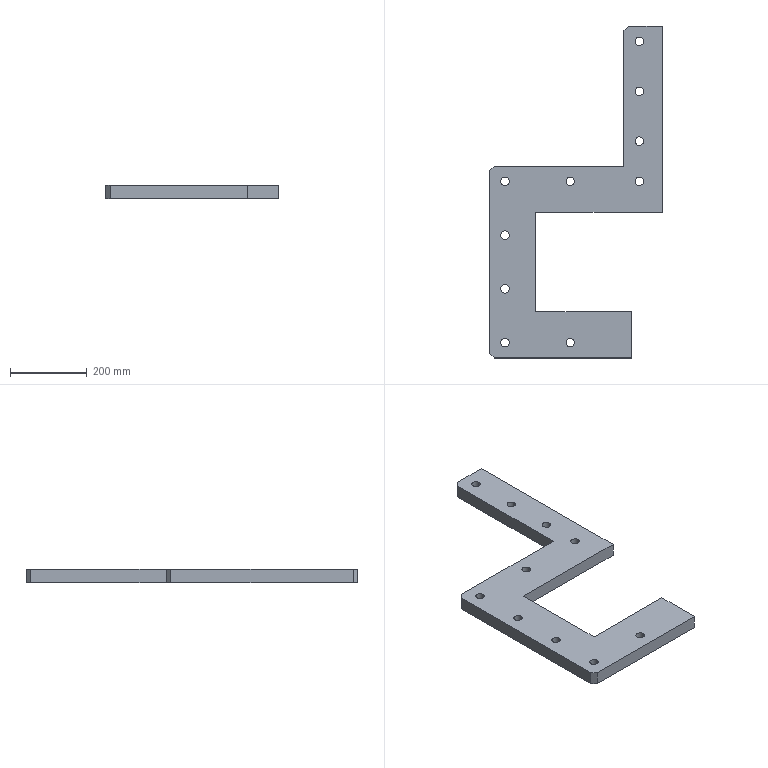Part | SolidWorks | features Chamfer 1, Extrusion 1, ICE 1 | 1 solid | 35 faces | box 450 x 865 x 35 mm | volume 5672894 mm3 | cylinder 20 | plane 15 | commonest cylinder face diameters 22 x20
STEP:
#1=CARTESIAN_POINT('',(-71.,-40.,0.));
#2=VERTEX_POINT('',#1);
#3=CARTESIAN_POINT('',(-49.,-40.,0.));
#4=VERTEX_POINT('',#3);
#5=CARTESIAN_POINT('',(-60.,-40.,0.));
#6=DIRECTION('',(0.,0.,1.));
#7=DIRECTION('',(1.,0.,0.));
#8=AXIS2_PLACEMENT_3D('',#5,#6,#7);
#9=CIRCLE('',#8,11.);
#10=EDGE_CURVE('',#2,#4,#9,.T.);
#11=ORIENTED_EDGE('',*,*,#10,.F.);
#12=CARTESIAN_POINT('',(-71.,-40.,35.));
#13=VERTEX_POINT('',#12);
#14=CARTESIAN_POINT('',(-71.,-40.,0.));
#15=DIRECTION('',(0.,0.,1.));
#16=VECTOR('',#15,1000.);
#17=LINE('',#14,#16);
#18=EDGE_CURVE('',#2,#13,#17,.T.);
#19=ORIENTED_EDGE('',*,*,#18,.T.);
#20=CARTESIAN_POINT('',(-49.,-40.,35.));
#21=VERTEX_POINT('',#20);
#22=CARTESIAN_POINT('',(-60.,-40.,35.));
#23=DIRECTION('',(0.,0.,1.));
#24=DIRECTION('',(1.,0.,0.));
#25=AXIS2_PLACEMENT_3D('',#22,#23,#24);
#26=CIRCLE('',#25,11.);
#27=EDGE_CURVE('',#13,#21,#26,.T.);
#28=ORIENTED_EDGE('',*,*,#27,.T.);
#29=CARTESIAN_POINT('',(-49.,-40.,0.));
#30=DIRECTION('',(0.,0.,1.));
#31=VECTOR('',#30,1000.);
#32=LINE('',#29,#31);
#33=EDGE_CURVE('',#4,#21,#32,.T.);
#34=ORIENTED_EDGE('',*,*,#33,.F.);
#35=EDGE_LOOP('',(#11,#19,#28,#34));
#36=FACE_OUTER_BOUND('',#35,.T.);
#37=CARTESIAN_POINT('',(-60.,-40.,0.));
#38=DIRECTION('',(0.,0.,1.));
#39=DIRECTION('',(1.,0.,0.));
#40=AXIS2_PLACEMENT_3D('',#37,#38,#39);
#41=CYLINDRICAL_SURFACE('',#40,11.);
#42=ADVANCED_FACE('',(#36),#41,.F.);
#43=CARTESIAN_POINT('',(-251.,-825.,0.));
#44=VERTEX_POINT('',#43);
#45=CARTESIAN_POINT('',(-229.,-825.,0.));
#46=VERTEX_POINT('',#45);
#47=CARTESIAN_POINT('',(-240.,-825.,0.));
#48=DIRECTION('',(0.,0.,1.));
#49=DIRECTION('',(1.,0.,0.));
#50=AXIS2_PLACEMENT_3D('',#47,#48,#49);
#51=CIRCLE('',#50,11.);
#52=EDGE_CURVE('',#44,#46,#51,.T.);
#53=ORIENTED_EDGE('',*,*,#52,.F.);
#54=CARTESIAN_POINT('',(-251.,-825.,35.));
#55=VERTEX_POINT('',#54);
#56=CARTESIAN_POINT('',(-251.,-825.,0.));
#57=DIRECTION('',(0.,0.,1.));
#58=VECTOR('',#57,1000.);
#59=LINE('',#56,#58);
#60=EDGE_CURVE('',#44,#55,#59,.T.);
#61=ORIENTED_EDGE('',*,*,#60,.T.);
#62=CARTESIAN_POINT('',(-229.,-825.,35.));
#63=VERTEX_POINT('',#62);
#64=CARTESIAN_POINT('',(-240.,-825.,35.));
#65=DIRECTION('',(0.,0.,1.));
#66=DIRECTION('',(1.,0.,0.));
#67=AXIS2_PLACEMENT_3D('',#64,#65,#66);
#68=CIRCLE('',#67,11.);
#69=EDGE_CURVE('',#55,#63,#68,.T.);
#70=ORIENTED_EDGE('',*,*,#69,.T.);
#71=CARTESIAN_POINT('',(-229.,-825.,0.));
#72=DIRECTION('',(0.,0.,1.));
#73=VECTOR('',#72,1000.);
#74=LINE('',#71,#73);
#75=EDGE_CURVE('',#46,#63,#74,.T.);
#76=ORIENTED_EDGE('',*,*,#75,.F.);
#77=EDGE_LOOP('',(#53,#61,#70,#76));
#78=FACE_OUTER_BOUND('',#77,.T.);
#79=CARTESIAN_POINT('',(-240.,-825.,0.));
#80=DIRECTION('',(0.,0.,1.));
#81=DIRECTION('',(1.,0.,0.));
#82=AXIS2_PLACEMENT_3D('',#79,#80,#81);
#83=CYLINDRICAL_SURFACE('',#82,11.);
#84=ADVANCED_FACE('',(#78),#83,.F.);
#85=CARTESIAN_POINT('',(-421.,-825.,0.));
#86=VERTEX_POINT('',#85);
#87=CARTESIAN_POINT('',(-399.,-825.,0.));
#88=VERTEX_POINT('',#87);
#89=CARTESIAN_POINT('',(-410.,-825.,0.));
#90=DIRECTION('',(0.,0.,1.));
#91=DIRECTION('',(1.,0.,0.));
#92=AXIS2_PLACEMENT_3D('',#89,#90,#91);
#93=CIRCLE('',#92,11.);
#94=EDGE_CURVE('',#86,#88,#93,.T.);
#95=ORIENTED_EDGE('',*,*,#94,.F.);
#96=CARTESIAN_POINT('',(-421.,-825.,35.));
#97=VERTEX_POINT('',#96);
#98=CARTESIAN_POINT('',(-421.,-825.,0.));
#99=DIRECTION('',(0.,0.,1.));
#100=VECTOR('',#99,1000.);
#101=LINE('',#98,#100);
#102=EDGE_CURVE('',#86,#97,#101,.T.);
#103=ORIENTED_EDGE('',*,*,#102,.T.);
#104=CARTESIAN_POINT('',(-399.,-825.,35.));
#105=VERTEX_POINT('',#104);
#106=CARTESIAN_POINT('',(-410.,-825.,35.));
#107=DIRECTION('',(0.,0.,1.));
#108=DIRECTION('',(1.,0.,0.));
#109=AXIS2_PLACEMENT_3D('',#106,#107,#108);
#110=CIRCLE('',#109,11.);
#111=EDGE_CURVE('',#97,#105,#110,.T.);
#112=ORIENTED_EDGE('',*,*,#111,.T.);
#113=CARTESIAN_POINT('',(-399.,-825.,0.));
#114=DIRECTION('',(0.,0.,1.));
#115=VECTOR('',#114,1000.);
#116=LINE('',#113,#115);
#117=EDGE_CURVE('',#88,#105,#116,.T.);
#118=ORIENTED_EDGE('',*,*,#117,.F.);
#119=EDGE_LOOP('',(#95,#103,#112,#118));
#120=FACE_OUTER_BOUND('',#119,.T.);
#121=CARTESIAN_POINT('',(-410.,-825.,0.));
#122=DIRECTION('',(0.,0.,1.));
#123=DIRECTION('',(1.,0.,0.));
#124=AXIS2_PLACEMENT_3D('',#121,#122,#123);
#125=CYLINDRICAL_SURFACE('',#124,11.);
#126=ADVANCED_FACE('',(#120),#125,.F.);
#127=CARTESIAN_POINT('',(-421.,-685.,0.));
#128=VERTEX_POINT('',#127);
#129=CARTESIAN_POINT('',(-399.,-685.,0.));
#130=VERTEX_POINT('',#129);
#131=CARTESIAN_POINT('',(-410.,-685.,0.));
#132=DIRECTION('',(0.,0.,1.));
#133=DIRECTION('',(1.,0.,0.));
#134=AXIS2_PLACEMENT_3D('',#131,#132,#133);
#135=CIRCLE('',#134,11.);
#136=EDGE_CURVE('',#128,#130,#135,.T.);
#137=ORIENTED_EDGE('',*,*,#136,.F.);
#138=CARTESIAN_POINT('',(-421.,-685.,35.));
#139=VERTEX_POINT('',#138);
#140=CARTESIAN_POINT('',(-421.,-685.,0.));
#141=DIRECTION('',(0.,0.,1.));
#142=VECTOR('',#141,1000.);
#143=LINE('',#140,#142);
#144=EDGE_CURVE('',#128,#139,#143,.T.);
#145=ORIENTED_EDGE('',*,*,#144,.T.);
#146=CARTESIAN_POINT('',(-399.,-685.,35.));
#147=VERTEX_POINT('',#146);
#148=CARTESIAN_POINT('',(-410.,-685.,35.));
#149=DIRECTION('',(0.,0.,1.));
#150=DIRECTION('',(1.,0.,0.));
#151=AXIS2_PLACEMENT_3D('',#148,#149,#150);
#152=CIRCLE('',#151,11.);
#153=EDGE_CURVE('',#139,#147,#152,.T.);
#154=ORIENTED_EDGE('',*,*,#153,.T.);
#155=CARTESIAN_POINT('',(-399.,-685.,0.));
#156=DIRECTION('',(0.,0.,1.));
#157=VECTOR('',#156,1000.);
#158=LINE('',#155,#157);
#159=EDGE_CURVE('',#130,#147,#158,.T.);
#160=ORIENTED_EDGE('',*,*,#159,.F.);
#161=EDGE_LOOP('',(#137,#145,#154,#160));
#162=FACE_OUTER_BOUND('',#161,.T.);
#163=CARTESIAN_POINT('',(-410.,-685.,0.));
#164=DIRECTION('',(0.,0.,1.));
#165=DIRECTION('',(1.,0.,0.));
#166=AXIS2_PLACEMENT_3D('',#163,#164,#165);
#167=CYLINDRICAL_SURFACE('',#166,11.);
#168=ADVANCED_FACE('',(#162),#167,.F.);
#169=CARTESIAN_POINT('',(-421.,-545.,0.));
#170=VERTEX_POINT('',#169);
#171=CARTESIAN_POINT('',(-399.,-545.,0.));
#172=VERTEX_POINT('',#171);
#173=CARTESIAN_POINT('',(-410.,-545.,0.));
#174=DIRECTION('',(0.,0.,1.));
#175=DIRECTION('',(1.,0.,0.));
#176=AXIS2_PLACEMENT_3D('',#173,#174,#175);
#177=CIRCLE('',#176,11.);
#178=EDGE_CURVE('',#170,#172,#177,.T.);
#179=ORIENTED_EDGE('',*,*,#178,.F.);
#180=CARTESIAN_POINT('',(-421.,-545.,35.));
#181=VERTEX_POINT('',#180);
#182=CARTESIAN_POINT('',(-421.,-545.,0.));
#183=DIRECTION('',(0.,0.,1.));
#184=VECTOR('',#183,1000.);
#185=LINE('',#182,#184);
#186=EDGE_CURVE('',#170,#181,#185,.T.);
#187=ORIENTED_EDGE('',*,*,#186,.T.);
#188=CARTESIAN_POINT('',(-399.,-545.,35.));
#189=VERTEX_POINT('',#188);
#190=CARTESIAN_POINT('',(-410.,-545.,35.));
#191=DIRECTION('',(0.,0.,1.));
#192=DIRECTION('',(1.,0.,0.));
#193=AXIS2_PLACEMENT_3D('',#190,#191,#192);
#194=CIRCLE('',#193,11.);
#195=EDGE_CURVE('',#181,#189,#194,.T.);
#196=ORIENTED_EDGE('',*,*,#195,.T.);
#197=CARTESIAN_POINT('',(-399.,-545.,0.));
#198=DIRECTION('',(0.,0.,1.));
#199=VECTOR('',#198,1000.);
#200=LINE('',#197,#199);
#201=EDGE_CURVE('',#172,#189,#200,.T.);
#202=ORIENTED_EDGE('',*,*,#201,.F.);
#203=EDGE_LOOP('',(#179,#187,#196,#202));
#204=FACE_OUTER_BOUND('',#203,.T.);
#205=CARTESIAN_POINT('',(-410.,-545.,0.));
#206=DIRECTION('',(0.,0.,1.));
#207=DIRECTION('',(1.,0.,0.));
#208=AXIS2_PLACEMENT_3D('',#205,#206,#207);
#209=CYLINDRICAL_SURFACE('',#208,11.);
#210=ADVANCED_FACE('',(#204),#209,.F.);
#211=CARTESIAN_POINT('',(-421.,-405.,0.));
#212=VERTEX_POINT('',#211);
#213=CARTESIAN_POINT('',(-399.,-405.,0.));
#214=VERTEX_POINT('',#213);
#215=CARTESIAN_POINT('',(-410.,-405.,0.));
#216=DIRECTION('',(0.,0.,1.));
#217=DIRECTION('',(1.,0.,0.));
#218=AXIS2_PLACEMENT_3D('',#215,#216,#217);
#219=CIRCLE('',#218,11.);
#220=EDGE_CURVE('',#212,#214,#219,.T.);
#221=ORIENTED_EDGE('',*,*,#220,.F.);
#222=CARTESIAN_POINT('',(-421.,-405.,35.));
#223=VERTEX_POINT('',#222);
#224=CARTESIAN_POINT('',(-421.,-405.,0.));
#225=DIRECTION('',(0.,0.,1.));
#226=VECTOR('',#225,1000.);
#227=LINE('',#224,#226);
#228=EDGE_CURVE('',#212,#223,#227,.T.);
#229=ORIENTED_EDGE('',*,*,#228,.T.);
#230=CARTESIAN_POINT('',(-399.,-405.,35.));
#231=VERTEX_POINT('',#230);
#232=CARTESIAN_POINT('',(-410.,-405.,35.));
#233=DIRECTION('',(0.,0.,1.));
#234=DIRECTION('',(1.,0.,0.));
#235=AXIS2_PLACEMENT_3D('',#232,#233,#234);
#236=CIRCLE('',#235,11.);
#237=EDGE_CURVE('',#223,#231,#236,.T.);
#238=ORIENTED_EDGE('',*,*,#237,.T.);
#239=CARTESIAN_POINT('',(-399.,-405.,0.));
#240=DIRECTION('',(0.,0.,1.));
#241=VECTOR('',#240,1000.);
#242=LINE('',#239,#241);
#243=EDGE_CURVE('',#214,#231,#242,.T.);
#244=ORIENTED_EDGE('',*,*,#243,.F.);
#245=EDGE_LOOP('',(#221,#229,#238,#244));
#246=FACE_OUTER_BOUND('',#245,.T.);
#247=CARTESIAN_POINT('',(-410.,-405.,0.));
#248=DIRECTION('',(0.,0.,1.));
#249=DIRECTION('',(1.,0.,0.));
#250=AXIS2_PLACEMENT_3D('',#247,#248,#249);
#251=CYLINDRICAL_SURFACE('',#250,11.);
#252=ADVANCED_FACE('',(#246),#251,.F.);
#253=CARTESIAN_POINT('',(-251.,-405.,0.));
#254=VERTEX_POINT('',#253);
#255=CARTESIAN_POINT('',(-229.,-405.,0.));
#256=VERTEX_POINT('',#255);
#257=CARTESIAN_POINT('',(-240.,-405.,0.));
#258=DIRECTION('',(0.,0.,1.));
#259=DIRECTION('',(1.,0.,0.));
#260=AXIS2_PLACEMENT_3D('',#257,#258,#259);
#261=CIRCLE('',#260,11.);
#262=EDGE_CURVE('',#254,#256,#261,.T.);
#263=ORIENTED_EDGE('',*,*,#262,.F.);
#264=CARTESIAN_POINT('',(-251.,-405.,35.));
#265=VERTEX_POINT('',#264);
#266=CARTESIAN_POINT('',(-251.,-405.,0.));
#267=DIRECTION('',(0.,0.,1.));
#268=VECTOR('',#267,1000.);
#269=LINE('',#266,#268);
#270=EDGE_CURVE('',#254,#265,#269,.T.);
#271=ORIENTED_EDGE('',*,*,#270,.T.);
#272=CARTESIAN_POINT('',(-229.,-405.,35.));
#273=VERTEX_POINT('',#272);
#274=CARTESIAN_POINT('',(-240.,-405.,35.));
#275=DIRECTION('',(0.,0.,1.));
#276=DIRECTION('',(1.,0.,0.));
#277=AXIS2_PLACEMENT_3D('',#274,#275,#276);
#278=CIRCLE('',#277,11.);
#279=EDGE_CURVE('',#265,#273,#278,.T.);
#280=ORIENTED_EDGE('',*,*,#279,.T.);
#281=CARTESIAN_POINT('',(-229.,-405.,0.));
#282=DIRECTION('',(0.,0.,1.));
#283=VECTOR('',#282,1000.);
#284=LINE('',#281,#283);
#285=EDGE_CURVE('',#256,#273,#284,.T.);
#286=ORIENTED_EDGE('',*,*,#285,.F.);
#287=EDGE_LOOP('',(#263,#271,#280,#286));
#288=FACE_OUTER_BOUND('',#287,.T.);
#289=CARTESIAN_POINT('',(-240.,-405.,0.));
#290=DIRECTION('',(0.,0.,1.));
#291=DIRECTION('',(1.,0.,0.));
#292=AXIS2_PLACEMENT_3D('',#289,#290,#291);
#293=CYLINDRICAL_SURFACE('',#292,11.);
#294=ADVANCED_FACE('',(#288),#293,.F.);
#295=CARTESIAN_POINT('',(-71.,-405.,0.));
#296=VERTEX_POINT('',#295);
#297=CARTESIAN_POINT('',(-49.,-405.,0.));
#298=VERTEX_POINT('',#297);
#299=CARTESIAN_POINT('',(-60.,-405.,0.));
#300=DIRECTION('',(0.,0.,1.));
#301=DIRECTION('',(1.,0.,0.));
#302=AXIS2_PLACEMENT_3D('',#299,#300,#301);
#303=CIRCLE('',#302,11.);
#304=EDGE_CURVE('',#296,#298,#303,.T.);
#305=ORIENTED_EDGE('',*,*,#304,.F.);
#306=CARTESIAN_POINT('',(-71.,-405.,35.));
#307=VERTEX_POINT('',#306);
#308=CARTESIAN_POINT('',(-71.,-405.,0.));
#309=DIRECTION('',(0.,0.,1.));
#310=VECTOR('',#309,1000.);
#311=LINE('',#308,#310);
#312=EDGE_CURVE('',#296,#307,#311,.T.);
#313=ORIENTED_EDGE('',*,*,#312,.T.);
#314=CARTESIAN_POINT('',(-49.,-405.,35.));
#315=VERTEX_POINT('',#314);
#316=CARTESIAN_POINT('',(-60.,-405.,35.));
#317=DIRECTION('',(0.,0.,1.));
#318=DIRECTION('',(1.,0.,0.));
#319=AXIS2_PLACEMENT_3D('',#316,#317,#318);
#320=CIRCLE('',#319,11.);
#321=EDGE_CURVE('',#307,#315,#320,.T.);
#322=ORIENTED_EDGE('',*,*,#321,.T.);
#323=CARTESIAN_POINT('',(-49.,-405.,0.));
#324=DIRECTION('',(0.,0.,1.));
#325=VECTOR('',#324,1000.);
#326=LINE('',#323,#325);
#327=EDGE_CURVE('',#298,#315,#326,.T.);
#328=ORIENTED_EDGE('',*,*,#327,.F.);
#329=EDGE_LOOP('',(#305,#313,#322,#328));
#330=FACE_OUTER_BOUND('',#329,.T.);
#331=CARTESIAN_POINT('',(-60.,-405.,0.));
#332=DIRECTION('',(0.,0.,1.));
#333=DIRECTION('',(1.,0.,0.));
#334=AXIS2_PLACEMENT_3D('',#331,#332,#333);
#335=CYLINDRICAL_SURFACE('',#334,11.);
#336=ADVANCED_FACE('',(#330),#335,.F.);
#337=CARTESIAN_POINT('',(-71.,-300.,0.));
#338=VERTEX_POINT('',#337);
#339=CARTESIAN_POINT('',(-49.,-300.,0.));
#340=VERTEX_POINT('',#339);
#341=CARTESIAN_POINT('',(-60.,-300.,0.));
#342=DIRECTION('',(0.,0.,1.));
#343=DIRECTION('',(1.,0.,0.));
#344=AXIS2_PLACEMENT_3D('',#341,#342,#343);
#345=CIRCLE('',#344,11.);
#346=EDGE_CURVE('',#338,#340,#345,.T.);
#347=ORIENTED_EDGE('',*,*,#346,.F.);
#348=CARTESIAN_POINT('',(-71.,-300.,35.));
#349=VERTEX_POINT('',#348);
#350=CARTESIAN_POINT('',(-71.,-300.,0.));
#351=DIRECTION('',(0.,0.,1.));
#352=VECTOR('',#351,1000.);
#353=LINE('',#350,#352);
#354=EDGE_CURVE('',#338,#349,#353,.T.);
#355=ORIENTED_EDGE('',*,*,#354,.T.);
#356=CARTESIAN_POINT('',(-49.,-300.,35.));
#357=VERTEX_POINT('',#356);
#358=CARTESIAN_POINT('',(-60.,-300.,35.));
#359=DIRECTION('',(0.,0.,1.));
#360=DIRECTION('',(1.,0.,0.));
#361=AXIS2_PLACEMENT_3D('',#358,#359,#360);
#362=CIRCLE('',#361,11.);
#363=EDGE_CURVE('',#349,#357,#362,.T.);
#364=ORIENTED_EDGE('',*,*,#363,.T.);
#365=CARTESIAN_POINT('',(-49.,-300.,0.));
#366=DIRECTION('',(0.,0.,1.));
#367=VECTOR('',#366,1000.);
#368=LINE('',#365,#367);
#369=EDGE_CURVE('',#340,#357,#368,.T.);
#370=ORIENTED_EDGE('',*,*,#369,.F.);
#371=EDGE_LOOP('',(#347,#355,#364,#370));
#372=FACE_OUTER_BOUND('',#371,.T.);
#373=CARTESIAN_POINT('',(-60.,-300.,0.));
#374=DIRECTION('',(0.,0.,1.));
#375=DIRECTION('',(1.,0.,0.));
#376=AXIS2_PLACEMENT_3D('',#373,#374,#375);
#377=CYLINDRICAL_SURFACE('',#376,11.);
#378=ADVANCED_FACE('',(#372),#377,.F.);
#379=CARTESIAN_POINT('',(-71.,-170.,0.));
#380=VERTEX_POINT('',#379);
#381=CARTESIAN_POINT('',(-49.,-170.,0.));
#382=VERTEX_POINT('',#381);
#383=CARTESIAN_POINT('',(-60.,-170.,0.));
#384=DIRECTION('',(0.,0.,1.));
#385=DIRECTION('',(1.,0.,0.));
#386=AXIS2_PLACEMENT_3D('',#383,#384,#385);
#387=CIRCLE('',#386,11.);
#388=EDGE_CURVE('',#380,#382,#387,.T.);
#389=ORIENTED_EDGE('',*,*,#388,.F.);
#390=CARTESIAN_POINT('',(-71.,-170.,35.));
#391=VERTEX_POINT('',#390);
#392=CARTESIAN_POINT('',(-71.,-170.,0.));
#393=DIRECTION('',(0.,0.,1.));
#394=VECTOR('',#393,1000.);
#395=LINE('',#392,#394);
#396=EDGE_CURVE('',#380,#391,#395,.T.);
#397=ORIENTED_EDGE('',*,*,#396,.T.);
#398=CARTESIAN_POINT('',(-49.,-170.,35.));
#399=VERTEX_POINT('',#398);
#400=CARTESIAN_POINT('',(-60.,-170.,35.));
#401=DIRECTION('',(0.,0.,1.));
#402=DIRECTION('',(1.,0.,0.));
#403=AXIS2_PLACEMENT_3D('',#400,#401,#402);
#404=CIRCLE('',#403,11.);
#405=EDGE_CURVE('',#391,#399,#404,.T.);
#406=ORIENTED_EDGE('',*,*,#405,.T.);
#407=CARTESIAN_POINT('',(-49.,-170.,0.));
#408=DIRECTION('',(0.,0.,1.));
#409=VECTOR('',#408,1000.);
#410=LINE('',#407,#409);
#411=EDGE_CURVE('',#382,#399,#410,.T.);
#412=ORIENTED_EDGE('',*,*,#411,.F.);
#413=EDGE_LOOP('',(#389,#397,#406,#412));
#414=FACE_OUTER_BOUND('',#413,.T.);
#415=CARTESIAN_POINT('',(-60.,-170.,0.));
#416=DIRECTION('',(0.,0.,1.));
#417=DIRECTION('',(1.,0.,0.));
#418=AXIS2_PLACEMENT_3D('',#415,#416,#417);
#419=CYLINDRICAL_SURFACE('',#418,11.);
#420=ADVANCED_FACE('',(#414),#419,.F.);
#421=CARTESIAN_POINT('',(-100.,-365.,0.));
#422=VERTEX_POINT('',#421);
#423=CARTESIAN_POINT('',(-438.,-365.,0.));
#424=VERTEX_POINT('',#423);
#425=CARTESIAN_POINT('',(-100.,-365.,0.));
#426=DIRECTION('',(-1.,0.,0.));
#427=VECTOR('',#426,1000.);
#428=LINE('',#425,#427);
#429=EDGE_CURVE('',#422,#424,#428,.T.);
#430=ORIENTED_EDGE('',*,*,#429,.T.);
#431=CARTESIAN_POINT('',(-438.,-365.,35.));
#432=VERTEX_POINT('',#431);
#433=CARTESIAN_POINT('',(-438.,-365.,35.));
#434=DIRECTION('',(0.,0.,1.));
#435=VECTOR('',#434,1000.);
#436=LINE('',#433,#435);
#437=EDGE_CURVE('',#424,#432,#436,.T.);
#438=ORIENTED_EDGE('',*,*,#437,.T.);
#439=CARTESIAN_POINT('',(-100.,-365.,35.));
#440=VERTEX_POINT('',#439);
#441=CARTESIAN_POINT('',(-100.,-365.,35.));
#442=DIRECTION('',(-1.,0.,0.));
#443=VECTOR('',#442,1000.);
#444=LINE('',#441,#443);
#445=EDGE_CURVE('',#440,#432,#444,.T.);
#446=ORIENTED_EDGE('',*,*,#445,.F.);
#447=CARTESIAN_POINT('',(-100.,-365.,35.));
#448=DIRECTION('',(0.,0.,-1.));
#449=VECTOR('',#448,1000.);
#450=LINE('',#447,#449);
#451=EDGE_CURVE('',#440,#422,#450,.T.);
#452=ORIENTED_EDGE('',*,*,#451,.T.);
#453=EDGE_LOOP('',(#430,#438,#446,#452));
#454=FACE_OUTER_BOUND('',#453,.T.);
#455=CARTESIAN_POINT('',(-100.,-365.,35.));
#456=DIRECTION('',(0.,-1.,0.));
#457=DIRECTION('',(1.,0.,0.));
#458=AXIS2_PLACEMENT_3D('',#455,#456,#457);
#459=PLANE('',#458);
#460=ADVANCED_FACE('',(#454),#459,.F.);
#461=CARTESIAN_POINT('',(-450.,-377.,0.));
#462=VERTEX_POINT('',#461);
#463=CARTESIAN_POINT('',(-450.,-853.,0.));
#464=VERTEX_POINT('',#463);
#465=CARTESIAN_POINT('',(-450.,-365.,0.));
#466=DIRECTION('',(0.,-1.,0.));
#467=VECTOR('',#466,1000.);
#468=LINE('',#465,#467);
#469=EDGE_CURVE('',#462,#464,#468,.T.);
#470=ORIENTED_EDGE('',*,*,#469,.T.);
#471=CARTESIAN_POINT('',(-450.,-853.,35.));
#472=VERTEX_POINT('',#471);
#473=CARTESIAN_POINT('',(-450.,-853.,35.));
#474=DIRECTION('',(0.,0.,1.));
#475=VECTOR('',#474,1000.);
#476=LINE('',#473,#475);
#477=EDGE_CURVE('',#464,#472,#476,.T.);
#478=ORIENTED_EDGE('',*,*,#477,.T.);
#479=CARTESIAN_POINT('',(-450.,-377.,35.));
#480=VERTEX_POINT('',#479);
#481=CARTESIAN_POINT('',(-450.,-365.,35.));
#482=DIRECTION('',(0.,-1.,0.));
#483=VECTOR('',#482,1000.);
#484=LINE('',#481,#483);
#485=EDGE_CURVE('',#480,#472,#484,.T.);
#486=ORIENTED_EDGE('',*,*,#485,.F.);
#487=CARTESIAN_POINT('',(-450.,-377.,35.));
#488=DIRECTION('',(0.,0.,-1.));
#489=VECTOR('',#488,1000.);
#490=LINE('',#487,#489);
#491=EDGE_CURVE('',#480,#462,#490,.T.);
#492=ORIENTED_EDGE('',*,*,#491,.T.);
#493=EDGE_LOOP('',(#470,#478,#486,#492));
#494=FACE_OUTER_BOUND('',#493,.T.);
#495=CARTESIAN_POINT('',(-450.,-365.,35.));
#496=DIRECTION('',(1.,0.,0.));
#497=DIRECTION('',(0.,1.,0.));
#498=AXIS2_PLACEMENT_3D('',#495,#496,#497);
#499=PLANE('',#498);
#500=ADVANCED_FACE('',(#494),#499,.F.);
#501=CARTESIAN_POINT('',(-438.,-865.,35.));
#502=VERTEX_POINT('',#501);
#503=CARTESIAN_POINT('',(-80.,-865.,35.));
#504=VERTEX_POINT('',#503);
#505=CARTESIAN_POINT('',(-450.,-865.,35.));
#506=DIRECTION('',(1.,0.,0.));
#507=VECTOR('',#506,1000.);
#508=LINE('',#505,#507);
#509=EDGE_CURVE('',#502,#504,#508,.T.);
#510=ORIENTED_EDGE('',*,*,#509,.F.);
#511=CARTESIAN_POINT('',(-438.,-865.,0.));
#512=VERTEX_POINT('',#511);
#513=CARTESIAN_POINT('',(-438.,-865.,35.));
#514=DIRECTION('',(0.,0.,-1.));
#515=VECTOR('',#514,1000.);
#516=LINE('',#513,#515);
#517=EDGE_CURVE('',#502,#512,#516,.T.);
#518=ORIENTED_EDGE('',*,*,#517,.T.);
#519=CARTESIAN_POINT('',(-80.,-865.,0.));
#520=VERTEX_POINT('',#519);
#521=CARTESIAN_POINT('',(-450.,-865.,0.));
#522=DIRECTION('',(1.,0.,0.));
#523=VECTOR('',#522,1000.);
#524=LINE('',#521,#523);
#525=EDGE_CURVE('',#512,#520,#524,.T.);
#526=ORIENTED_EDGE('',*,*,#525,.T.);
#527=CARTESIAN_POINT('',(-80.,-865.,35.));
#528=DIRECTION('',(0.,0.,-1.));
#529=VECTOR('',#528,1000.);
#530=LINE('',#527,#529);
#531=EDGE_CURVE('',#504,#520,#530,.T.);
#532=ORIENTED_EDGE('',*,*,#531,.F.);
#533=EDGE_LOOP('',(#510,#518,#526,#532));
#534=FACE_OUTER_BOUND('',#533,.T.);
#535=CARTESIAN_POINT('',(-450.,-865.,35.));
#536=DIRECTION('',(0.,1.,0.));
#537=DIRECTION('',(0.,0.,1.));
#538=AXIS2_PLACEMENT_3D('',#535,#536,#537);
#539=PLANE('',#538);
#540=ADVANCED_FACE('',(#534),#539,.F.);
#541=CARTESIAN_POINT('',(-80.,-745.,0.));
#542=VERTEX_POINT('',#541);
#543=CARTESIAN_POINT('',(-80.,-865.,0.));
#544=DIRECTION('',(0.,1.,0.));
#545=VECTOR('',#544,1000.);
#546=LINE('',#543,#545);
#547=EDGE_CURVE('',#520,#542,#546,.T.);
#548=ORIENTED_EDGE('',*,*,#547,.T.);
#549=CARTESIAN_POINT('',(-80.,-745.,35.));
#550=VERTEX_POINT('',#549);
#551=CARTESIAN_POINT('',(-80.,-745.,35.));
#552=DIRECTION('',(0.,0.,-1.));
#553=VECTOR('',#552,1000.);
#554=LINE('',#551,#553);
#555=EDGE_CURVE('',#550,#542,#554,.T.);
#556=ORIENTED_EDGE('',*,*,#555,.F.);
#557=CARTESIAN_POINT('',(-80.,-865.,35.));
#558=DIRECTION('',(0.,1.,0.));
#559=VECTOR('',#558,1000.);
#560=LINE('',#557,#559);
#561=EDGE_CURVE('',#504,#550,#560,.T.);
#562=ORIENTED_EDGE('',*,*,#561,.F.);
#563=ORIENTED_EDGE('',*,*,#531,.T.);
#564=EDGE_LOOP('',(#548,#556,#562,#563));
#565=FACE_OUTER_BOUND('',#564,.T.);
#566=CARTESIAN_POINT('',(-80.,-865.,35.));
#567=DIRECTION('',(-1.,0.,0.));
#568=DIRECTION('',(0.,0.,1.));
#569=AXIS2_PLACEMENT_3D('',#566,#567,#568);
#570=PLANE('',#569);
#571=ADVANCED_FACE('',(#565),#570,.F.);
#572=CARTESIAN_POINT('',(-330.,-745.,0.));
#573=VERTEX_POINT('',#572);
#574=CARTESIAN_POINT('',(-330.,-745.,0.));
#575=DIRECTION('',(-1.,0.,0.));
#576=VECTOR('',#575,1000.);
#577=LINE('',#574,#576);
#578=EDGE_CURVE('',#542,#573,#577,.T.);
#579=ORIENTED_EDGE('',*,*,#578,.T.);
#580=CARTESIAN_POINT('',(-330.,-745.,35.));
#581=VERTEX_POINT('',#580);
#582=CARTESIAN_POINT('',(-330.,-745.,35.));
#583=DIRECTION('',(0.,0.,-1.));
#584=VECTOR('',#583,1000.);
#585=LINE('',#582,#584);
#586=EDGE_CURVE('',#581,#573,#585,.T.);
#587=ORIENTED_EDGE('',*,*,#586,.F.);
#588=CARTESIAN_POINT('',(-330.,-745.,35.));
#589=DIRECTION('',(-1.,0.,0.));
#590=VECTOR('',#589,1000.);
#591=LINE('',#588,#590);
#592=EDGE_CURVE('',#550,#581,#591,.T.);
#593=ORIENTED_EDGE('',*,*,#592,.F.);
#594=ORIENTED_EDGE('',*,*,#555,.T.);
#595=EDGE_LOOP('',(#579,#587,#593,#594));
#596=FACE_OUTER_BOUND('',#595,.T.);
#597=CARTESIAN_POINT('',(-330.,-745.,35.));
#598=DIRECTION('',(0.,-1.,0.));
#599=DIRECTION('',(0.,0.,-1.));
#600=AXIS2_PLACEMENT_3D('',#597,#598,#599);
#601=PLANE('',#600);
#602=ADVANCED_FACE('',(#596),#601,.F.);
#603=CARTESIAN_POINT('',(-330.,-485.,0.));
#604=VERTEX_POINT('',#603);
#605=CARTESIAN_POINT('',(-330.,-485.,0.));
#606=DIRECTION('',(0.,1.,0.));
#607=VECTOR('',#606,1000.);
#608=LINE('',#605,#607);
#609=EDGE_CURVE('',#573,#604,#608,.T.);
#610=ORIENTED_EDGE('',*,*,#609,.T.);
#611=CARTESIAN_POINT('',(-330.,-485.,35.));
#612=VERTEX_POINT('',#611);
#613=CARTESIAN_POINT('',(-330.,-485.,35.));
#614=DIRECTION('',(0.,0.,-1.));
#615=VECTOR('',#614,1000.);
#616=LINE('',#613,#615);
#617=EDGE_CURVE('',#612,#604,#616,.T.);
#618=ORIENTED_EDGE('',*,*,#617,.F.);
#619=CARTESIAN_POINT('',(-330.,-485.,35.));
#620=DIRECTION('',(0.,1.,0.));
#621=VECTOR('',#620,1000.);
#622=LINE('',#619,#621);
#623=EDGE_CURVE('',#581,#612,#622,.T.);
#624=ORIENTED_EDGE('',*,*,#623,.F.);
#625=ORIENTED_EDGE('',*,*,#586,.T.);
#626=EDGE_LOOP('',(#610,#618,#624,#625));
#627=FACE_OUTER_BOUND('',#626,.T.);
#628=CARTESIAN_POINT('',(-330.,-485.,35.));
#629=DIRECTION('',(-1.,0.,0.));
#630=DIRECTION('',(0.,-1.,0.));
#631=AXIS2_PLACEMENT_3D('',#628,#629,#630);
#632=PLANE('',#631);
#633=ADVANCED_FACE('',(#627),#632,.F.);
#634=CARTESIAN_POINT('',(0.,-485.,0.));
#635=VERTEX_POINT('',#634);
#636=CARTESIAN_POINT('',(0.,-485.,0.));
#637=DIRECTION('',(1.,0.,0.));
#638=VECTOR('',#637,1000.);
#639=LINE('',#636,#638);
#640=EDGE_CURVE('',#604,#635,#639,.T.);
#641=ORIENTED_EDGE('',*,*,#640,.T.);
#642=CARTESIAN_POINT('',(0.,-485.,35.));
#643=VERTEX_POINT('',#642);
#644=CARTESIAN_POINT('',(0.,-485.,35.));
#645=DIRECTION('',(0.,0.,-1.));
#646=VECTOR('',#645,1000.);
#647=LINE('',#644,#646);
#648=EDGE_CURVE('',#643,#635,#647,.T.);
#649=ORIENTED_EDGE('',*,*,#648,.F.);
#650=CARTESIAN_POINT('',(0.,-485.,35.));
#651=DIRECTION('',(1.,0.,0.));
#652=VECTOR('',#651,1000.);
#653=LINE('',#650,#652);
#654=EDGE_CURVE('',#612,#643,#653,.T.);
#655=ORIENTED_EDGE('',*,*,#654,.F.);
#656=ORIENTED_EDGE('',*,*,#617,.T.);
#657=EDGE_LOOP('',(#641,#649,#655,#656));
#658=FACE_OUTER_BOUND('',#657,.T.);
#659=CARTESIAN_POINT('',(0.,-485.,35.));
#660=DIRECTION('',(0.,1.,0.));
#661=DIRECTION('',(-1.,0.,0.));
#662=AXIS2_PLACEMENT_3D('',#659,#660,#661);
#663=PLANE('',#662);
#664=ADVANCED_FACE('',(#658),#663,.F.);
#665=CARTESIAN_POINT('',(0.,0.,0.));
#666=VERTEX_POINT('',#665);
#667=CARTESIAN_POINT('',(0.,0.,0.));
#668=DIRECTION('',(0.,1.,0.));
#669=VECTOR('',#668,1000.);
#670=LINE('',#667,#669);
#671=EDGE_CURVE('',#635,#666,#670,.T.);
#672=ORIENTED_EDGE('',*,*,#671,.T.);
#673=CARTESIAN_POINT('',(0.,0.,35.));
#674=VERTEX_POINT('',#673);
#675=CARTESIAN_POINT('',(0.,0.,35.));
#676=DIRECTION('',(0.,0.,-1.));
#677=VECTOR('',#676,1000.);
#678=LINE('',#675,#677);
#679=EDGE_CURVE('',#674,#666,#678,.T.);
#680=ORIENTED_EDGE('',*,*,#679,.F.);
#681=CARTESIAN_POINT('',(0.,0.,35.));
#682=DIRECTION('',(0.,1.,0.));
#683=VECTOR('',#682,1000.);
#684=LINE('',#681,#683);
#685=EDGE_CURVE('',#643,#674,#684,.T.);
#686=ORIENTED_EDGE('',*,*,#685,.F.);
#687=ORIENTED_EDGE('',*,*,#648,.T.);
#688=EDGE_LOOP('',(#672,#680,#686,#687));
#689=FACE_OUTER_BOUND('',#688,.T.);
#690=CARTESIAN_POINT('',(0.,0.,35.));
#691=DIRECTION('',(-1.,0.,0.));
#692=DIRECTION('',(0.,-1.,0.));
#693=AXIS2_PLACEMENT_3D('',#690,#691,#692);
#694=PLANE('',#693);
#695=ADVANCED_FACE('',(#689),#694,.F.);
#696=CARTESIAN_POINT('',(-88.,0.,0.));
#697=VERTEX_POINT('',#696);
#698=CARTESIAN_POINT('',(0.,0.,0.));
#699=DIRECTION('',(-1.,0.,0.));
#700=VECTOR('',#699,1000.);
#701=LINE('',#698,#700);
#702=EDGE_CURVE('',#666,#697,#701,.T.);
#703=ORIENTED_EDGE('',*,*,#702,.T.);
#704=CARTESIAN_POINT('',(-88.,0.,35.));
#705=VERTEX_POINT('',#704);
#706=CARTESIAN_POINT('',(-88.,0.,35.));
#707=DIRECTION('',(0.,0.,1.));
#708=VECTOR('',#707,1000.);
#709=LINE('',#706,#708);
#710=EDGE_CURVE('',#697,#705,#709,.T.);
#711=ORIENTED_EDGE('',*,*,#710,.T.);
#712=CARTESIAN_POINT('',(0.,0.,35.));
#713=DIRECTION('',(-1.,0.,0.));
#714=VECTOR('',#713,1000.);
#715=LINE('',#712,#714);
#716=EDGE_CURVE('',#674,#705,#715,.T.);
#717=ORIENTED_EDGE('',*,*,#716,.F.);
#718=ORIENTED_EDGE('',*,*,#679,.T.);
#719=EDGE_LOOP('',(#703,#711,#717,#718));
#720=FACE_OUTER_BOUND('',#719,.T.);
#721=CARTESIAN_POINT('',(0.,0.,35.));
#722=DIRECTION('',(0.,-1.,0.));
#723=DIRECTION('',(0.,0.,-1.));
#724=AXIS2_PLACEMENT_3D('',#721,#722,#723);
#725=PLANE('',#724);
#726=ADVANCED_FACE('',(#720),#725,.F.);
#727=CARTESIAN_POINT('',(-100.,-12.,35.));
#728=VERTEX_POINT('',#727);
#729=CARTESIAN_POINT('',(-100.,0.,35.));
#730=DIRECTION('',(0.,-1.,0.));
#731=VECTOR('',#730,1000.);
#732=LINE('',#729,#731);
#733=EDGE_CURVE('',#728,#440,#732,.T.);
#734=ORIENTED_EDGE('',*,*,#733,.F.);
#735=CARTESIAN_POINT('',(-100.,-12.,0.));
#736=VERTEX_POINT('',#735);
#737=CARTESIAN_POINT('',(-100.,-12.,35.));
#738=DIRECTION('',(0.,0.,-1.));
#739=VECTOR('',#738,1000.);
#740=LINE('',#737,#739);
#741=EDGE_CURVE('',#728,#736,#740,.T.);
#742=ORIENTED_EDGE('',*,*,#741,.T.);
#743=CARTESIAN_POINT('',(-100.,0.,0.));
#744=DIRECTION('',(0.,-1.,0.));
#745=VECTOR('',#744,1000.);
#746=LINE('',#743,#745);
#747=EDGE_CURVE('',#736,#422,#746,.T.);
#748=ORIENTED_EDGE('',*,*,#747,.T.);
#749=ORIENTED_EDGE('',*,*,#451,.F.);
#750=EDGE_LOOP('',(#734,#742,#748,#749));
#751=FACE_OUTER_BOUND('',#750,.T.);
#752=CARTESIAN_POINT('',(-100.,0.,35.));
#753=DIRECTION('',(1.,0.,0.));
#754=DIRECTION('',(0.,1.,0.));
#755=AXIS2_PLACEMENT_3D('',#752,#753,#754);
#756=PLANE('',#755);
#757=ADVANCED_FACE('',(#751),#756,.F.);
#758=CARTESIAN_POINT('',(-60.,-40.,35.));
#759=DIRECTION('',(0.,0.,1.));
#760=DIRECTION('',(1.,0.,0.));
#761=AXIS2_PLACEMENT_3D('',#758,#759,#760);
#762=CIRCLE('',#761,11.);
#763=EDGE_CURVE('',#21,#13,#762,.T.);
#764=ORIENTED_EDGE('',*,*,#763,.F.);
#765=ORIENTED_EDGE('',*,*,#27,.F.);
#766=EDGE_LOOP('',(#764,#765));
#767=FACE_BOUND('',#766,.T.);
#768=CARTESIAN_POINT('',(-240.,-825.,35.));
#769=DIRECTION('',(0.,0.,1.));
#770=DIRECTION('',(1.,0.,0.));
#771=AXIS2_PLACEMENT_3D('',#768,#769,#770);
#772=CIRCLE('',#771,11.);
#773=EDGE_CURVE('',#63,#55,#772,.T.);
#774=ORIENTED_EDGE('',*,*,#773,.F.);
#775=ORIENTED_EDGE('',*,*,#69,.F.);
#776=EDGE_LOOP('',(#774,#775));
#777=FACE_BOUND('',#776,.T.);
#778=CARTESIAN_POINT('',(-410.,-825.,35.));
#779=DIRECTION('',(0.,0.,1.));
#780=DIRECTION('',(1.,0.,0.));
#781=AXIS2_PLACEMENT_3D('',#778,#779,#780);
#782=CIRCLE('',#781,11.);
#783=EDGE_CURVE('',#105,#97,#782,.T.);
#784=ORIENTED_EDGE('',*,*,#783,.F.);
#785=ORIENTED_EDGE('',*,*,#111,.F.);
#786=EDGE_LOOP('',(#784,#785));
#787=FACE_BOUND('',#786,.T.);
#788=CARTESIAN_POINT('',(-410.,-685.,35.));
#789=DIRECTION('',(0.,0.,1.));
#790=DIRECTION('',(1.,0.,0.));
#791=AXIS2_PLACEMENT_3D('',#788,#789,#790);
#792=CIRCLE('',#791,11.);
#793=EDGE_CURVE('',#147,#139,#792,.T.);
#794=ORIENTED_EDGE('',*,*,#793,.F.);
#795=ORIENTED_EDGE('',*,*,#153,.F.);
#796=EDGE_LOOP('',(#794,#795));
#797=FACE_BOUND('',#796,.T.);
#798=CARTESIAN_POINT('',(-410.,-545.,35.));
#799=DIRECTION('',(0.,0.,1.));
#800=DIRECTION('',(1.,0.,0.));
#801=AXIS2_PLACEMENT_3D('',#798,#799,#800);
#802=CIRCLE('',#801,11.);
#803=EDGE_CURVE('',#189,#181,#802,.T.);
#804=ORIENTED_EDGE('',*,*,#803,.F.);
#805=ORIENTED_EDGE('',*,*,#195,.F.);
#806=EDGE_LOOP('',(#804,#805));
#807=FACE_BOUND('',#806,.T.);
#808=CARTESIAN_POINT('',(-410.,-405.,35.));
#809=DIRECTION('',(0.,0.,1.));
#810=DIRECTION('',(1.,0.,0.));
#811=AXIS2_PLACEMENT_3D('',#808,#809,#810);
#812=CIRCLE('',#811,11.);
#813=EDGE_CURVE('',#231,#223,#812,.T.);
#814=ORIENTED_EDGE('',*,*,#813,.F.);
#815=ORIENTED_EDGE('',*,*,#237,.F.);
#816=EDGE_LOOP('',(#814,#815));
#817=FACE_BOUND('',#816,.T.);
#818=CARTESIAN_POINT('',(-240.,-405.,35.));
#819=DIRECTION('',(0.,0.,1.));
#820=DIRECTION('',(1.,0.,0.));
#821=AXIS2_PLACEMENT_3D('',#818,#819,#820);
#822=CIRCLE('',#821,11.);
#823=EDGE_CURVE('',#273,#265,#822,.T.);
#824=ORIENTED_EDGE('',*,*,#823,.F.);
#825=ORIENTED_EDGE('',*,*,#279,.F.);
#826=EDGE_LOOP('',(#824,#825));
#827=FACE_BOUND('',#826,.T.);
#828=CARTESIAN_POINT('',(-60.,-405.,35.));
#829=DIRECTION('',(0.,0.,1.));
#830=DIRECTION('',(1.,0.,0.));
#831=AXIS2_PLACEMENT_3D('',#828,#829,#830);
#832=CIRCLE('',#831,11.);
#833=EDGE_CURVE('',#315,#307,#832,.T.);
#834=ORIENTED_EDGE('',*,*,#833,.F.);
#835=ORIENTED_EDGE('',*,*,#321,.F.);
#836=EDGE_LOOP('',(#834,#835));
#837=FACE_BOUND('',#836,.T.);
#838=CARTESIAN_POINT('',(-60.,-300.,35.));
#839=DIRECTION('',(0.,0.,1.));
#840=DIRECTION('',(1.,0.,0.));
#841=AXIS2_PLACEMENT_3D('',#838,#839,#840);
#842=CIRCLE('',#841,11.);
#843=EDGE_CURVE('',#357,#349,#842,.T.);
#844=ORIENTED_EDGE('',*,*,#843,.F.);
#845=ORIENTED_EDGE('',*,*,#363,.F.);
#846=EDGE_LOOP('',(#844,#845));
#847=FACE_BOUND('',#846,.T.);
#848=CARTESIAN_POINT('',(-60.,-170.,35.));
#849=DIRECTION('',(0.,0.,1.));
#850=DIRECTION('',(1.,0.,0.));
#851=AXIS2_PLACEMENT_3D('',#848,#849,#850);
#852=CIRCLE('',#851,11.);
#853=EDGE_CURVE('',#399,#391,#852,.T.);
#854=ORIENTED_EDGE('',*,*,#853,.F.);
#855=ORIENTED_EDGE('',*,*,#405,.F.);
#856=EDGE_LOOP('',(#854,#855));
#857=FACE_BOUND('',#856,.T.);
#858=ORIENTED_EDGE('',*,*,#485,.T.);
#859=CARTESIAN_POINT('',(-651.5,-651.5,35.));
#860=DIRECTION('',(0.7071,-0.7071,0.));
#861=VECTOR('',#860,1000.);
#862=LINE('',#859,#861);
#863=EDGE_CURVE('',#472,#502,#862,.T.);
#864=ORIENTED_EDGE('',*,*,#863,.T.);
#865=ORIENTED_EDGE('',*,*,#509,.T.);
#866=ORIENTED_EDGE('',*,*,#561,.T.);
#867=ORIENTED_EDGE('',*,*,#592,.T.);
#868=ORIENTED_EDGE('',*,*,#623,.T.);
#869=ORIENTED_EDGE('',*,*,#654,.T.);
#870=ORIENTED_EDGE('',*,*,#685,.T.);
#871=ORIENTED_EDGE('',*,*,#716,.T.);
#872=CARTESIAN_POINT('',(-44.,44.,35.));
#873=DIRECTION('',(-0.7071,-0.7071,0.));
#874=VECTOR('',#873,1000.);
#875=LINE('',#872,#874);
#876=EDGE_CURVE('',#705,#728,#875,.T.);
#877=ORIENTED_EDGE('',*,*,#876,.T.);
#878=ORIENTED_EDGE('',*,*,#733,.T.);
#879=ORIENTED_EDGE('',*,*,#445,.T.);
#880=CARTESIAN_POINT('',(-36.5,36.5,35.));
#881=DIRECTION('',(-0.7071,-0.7071,0.));
#882=VECTOR('',#881,1000.);
#883=LINE('',#880,#882);
#884=EDGE_CURVE('',#432,#480,#883,.T.);
#885=ORIENTED_EDGE('',*,*,#884,.T.);
#886=EDGE_LOOP('',(#858,#864,#865,#866,#867,#868,#869,#870,#871,#877,#878,#879,#885));
#887=FACE_OUTER_BOUND('',#886,.T.);
#888=CARTESIAN_POINT('',(0.,0.,35.));
#889=DIRECTION('',(0.,0.,1.));
#890=DIRECTION('',(1.,0.,0.));
#891=AXIS2_PLACEMENT_3D('',#888,#889,#890);
#892=PLANE('',#891);
#893=ADVANCED_FACE('',(#767,#777,#787,#797,#807,#817,#827,#837,#847,#857,#887),#892,.T.);
#894=CARTESIAN_POINT('',(-60.,-40.,0.));
#895=DIRECTION('',(0.,0.,1.));
#896=DIRECTION('',(1.,0.,0.));
#897=AXIS2_PLACEMENT_3D('',#894,#895,#896);
#898=CIRCLE('',#897,11.);
#899=EDGE_CURVE('',#4,#2,#898,.T.);
#900=ORIENTED_EDGE('',*,*,#899,.T.);
#901=ORIENTED_EDGE('',*,*,#10,.T.);
#902=EDGE_LOOP('',(#900,#901));
#903=FACE_BOUND('',#902,.T.);
#904=CARTESIAN_POINT('',(-240.,-825.,0.));
#905=DIRECTION('',(0.,0.,1.));
#906=DIRECTION('',(1.,0.,0.));
#907=AXIS2_PLACEMENT_3D('',#904,#905,#906);
#908=CIRCLE('',#907,11.);
#909=EDGE_CURVE('',#46,#44,#908,.T.);
#910=ORIENTED_EDGE('',*,*,#909,.T.);
#911=ORIENTED_EDGE('',*,*,#52,.T.);
#912=EDGE_LOOP('',(#910,#911));
#913=FACE_BOUND('',#912,.T.);
#914=CARTESIAN_POINT('',(-410.,-825.,0.));
#915=DIRECTION('',(0.,0.,1.));
#916=DIRECTION('',(1.,0.,0.));
#917=AXIS2_PLACEMENT_3D('',#914,#915,#916);
#918=CIRCLE('',#917,11.);
#919=EDGE_CURVE('',#88,#86,#918,.T.);
#920=ORIENTED_EDGE('',*,*,#919,.T.);
#921=ORIENTED_EDGE('',*,*,#94,.T.);
#922=EDGE_LOOP('',(#920,#921));
#923=FACE_BOUND('',#922,.T.);
#924=CARTESIAN_POINT('',(-410.,-685.,0.));
#925=DIRECTION('',(0.,0.,1.));
#926=DIRECTION('',(1.,0.,0.));
#927=AXIS2_PLACEMENT_3D('',#924,#925,#926);
#928=CIRCLE('',#927,11.);
#929=EDGE_CURVE('',#130,#128,#928,.T.);
#930=ORIENTED_EDGE('',*,*,#929,.T.);
#931=ORIENTED_EDGE('',*,*,#136,.T.);
#932=EDGE_LOOP('',(#930,#931));
#933=FACE_BOUND('',#932,.T.);
#934=CARTESIAN_POINT('',(-410.,-545.,0.));
#935=DIRECTION('',(0.,0.,1.));
#936=DIRECTION('',(1.,0.,0.));
#937=AXIS2_PLACEMENT_3D('',#934,#935,#936);
#938=CIRCLE('',#937,11.);
#939=EDGE_CURVE('',#172,#170,#938,.T.);
#940=ORIENTED_EDGE('',*,*,#939,.T.);
#941=ORIENTED_EDGE('',*,*,#178,.T.);
#942=EDGE_LOOP('',(#940,#941));
#943=FACE_BOUND('',#942,.T.);
#944=CARTESIAN_POINT('',(-410.,-405.,0.));
#945=DIRECTION('',(0.,0.,1.));
#946=DIRECTION('',(1.,0.,0.));
#947=AXIS2_PLACEMENT_3D('',#944,#945,#946);
#948=CIRCLE('',#947,11.);
#949=EDGE_CURVE('',#214,#212,#948,.T.);
#950=ORIENTED_EDGE('',*,*,#949,.T.);
#951=ORIENTED_EDGE('',*,*,#220,.T.);
#952=EDGE_LOOP('',(#950,#951));
#953=FACE_BOUND('',#952,.T.);
#954=CARTESIAN_POINT('',(-240.,-405.,0.));
#955=DIRECTION('',(0.,0.,1.));
#956=DIRECTION('',(1.,0.,0.));
#957=AXIS2_PLACEMENT_3D('',#954,#955,#956);
#958=CIRCLE('',#957,11.);
#959=EDGE_CURVE('',#256,#254,#958,.T.);
#960=ORIENTED_EDGE('',*,*,#959,.T.);
#961=ORIENTED_EDGE('',*,*,#262,.T.);
#962=EDGE_LOOP('',(#960,#961));
#963=FACE_BOUND('',#962,.T.);
#964=CARTESIAN_POINT('',(-60.,-405.,0.));
#965=DIRECTION('',(0.,0.,1.));
#966=DIRECTION('',(1.,0.,0.));
#967=AXIS2_PLACEMENT_3D('',#964,#965,#966);
#968=CIRCLE('',#967,11.);
#969=EDGE_CURVE('',#298,#296,#968,.T.);
#970=ORIENTED_EDGE('',*,*,#969,.T.);
#971=ORIENTED_EDGE('',*,*,#304,.T.);
#972=EDGE_LOOP('',(#970,#971));
#973=FACE_BOUND('',#972,.T.);
#974=CARTESIAN_POINT('',(-60.,-300.,0.));
#975=DIRECTION('',(0.,0.,1.));
#976=DIRECTION('',(1.,0.,0.));
#977=AXIS2_PLACEMENT_3D('',#974,#975,#976);
#978=CIRCLE('',#977,11.);
#979=EDGE_CURVE('',#340,#338,#978,.T.);
#980=ORIENTED_EDGE('',*,*,#979,.T.);
#981=ORIENTED_EDGE('',*,*,#346,.T.);
#982=EDGE_LOOP('',(#980,#981));
#983=FACE_BOUND('',#982,.T.);
#984=CARTESIAN_POINT('',(-60.,-170.,0.));
#985=DIRECTION('',(0.,0.,1.));
#986=DIRECTION('',(1.,0.,0.));
#987=AXIS2_PLACEMENT_3D('',#984,#985,#986);
#988=CIRCLE('',#987,11.);
#989=EDGE_CURVE('',#382,#380,#988,.T.);
#990=ORIENTED_EDGE('',*,*,#989,.T.);
#991=ORIENTED_EDGE('',*,*,#388,.T.);
#992=EDGE_LOOP('',(#990,#991));
#993=FACE_BOUND('',#992,.T.);
#994=ORIENTED_EDGE('',*,*,#525,.F.);
#995=CARTESIAN_POINT('',(-438.,-865.,0.));
#996=DIRECTION('',(-0.7071,0.7071,0.));
#997=VECTOR('',#996,1000.);
#998=LINE('',#995,#997);
#999=EDGE_CURVE('',#512,#464,#998,.T.);
#1000=ORIENTED_EDGE('',*,*,#999,.T.);
#1001=ORIENTED_EDGE('',*,*,#469,.F.);
#1002=CARTESIAN_POINT('',(-450.,-377.,0.));
#1003=DIRECTION('',(0.7071,0.7071,0.));
#1004=VECTOR('',#1003,1000.);
#1005=LINE('',#1002,#1004);
#1006=EDGE_CURVE('',#462,#424,#1005,.T.);
#1007=ORIENTED_EDGE('',*,*,#1006,.T.);
#1008=ORIENTED_EDGE('',*,*,#429,.F.);
#1009=ORIENTED_EDGE('',*,*,#747,.F.);
#1010=CARTESIAN_POINT('',(-100.,-12.,0.));
#1011=DIRECTION('',(0.7071,0.7071,0.));
#1012=VECTOR('',#1011,1000.);
#1013=LINE('',#1010,#1012);
#1014=EDGE_CURVE('',#736,#697,#1013,.T.);
#1015=ORIENTED_EDGE('',*,*,#1014,.T.);
#1016=ORIENTED_EDGE('',*,*,#702,.F.);
#1017=ORIENTED_EDGE('',*,*,#671,.F.);
#1018=ORIENTED_EDGE('',*,*,#640,.F.);
#1019=ORIENTED_EDGE('',*,*,#609,.F.);
#1020=ORIENTED_EDGE('',*,*,#578,.F.);
#1021=ORIENTED_EDGE('',*,*,#547,.F.);
#1022=EDGE_LOOP('',(#994,#1000,#1001,#1007,#1008,#1009,#1015,#1016,#1017,#1018,#1019,#1020,#1021));
#1023=FACE_OUTER_BOUND('',#1022,.T.);
#1024=CARTESIAN_POINT('',(0.,0.,0.));
#1025=DIRECTION('',(0.,0.,1.));
#1026=DIRECTION('',(1.,0.,0.));
#1027=AXIS2_PLACEMENT_3D('',#1024,#1025,#1026);
#1028=PLANE('',#1027);
#1029=ADVANCED_FACE('',(#903,#913,#923,#933,#943,#953,#963,#973,#983,#993,#1023),#1028,.F.);
#1030=ORIENTED_EDGE('',*,*,#863,.F.);
#1031=ORIENTED_EDGE('',*,*,#477,.F.);
#1032=ORIENTED_EDGE('',*,*,#999,.F.);
#1033=ORIENTED_EDGE('',*,*,#517,.F.);
#1034=EDGE_LOOP('',(#1030,#1031,#1032,#1033));
#1035=FACE_OUTER_BOUND('',#1034,.T.);
#1036=CARTESIAN_POINT('',(-438.,-865.,35.));
#1037=DIRECTION('',(0.7071,0.7071,0.));
#1038=DIRECTION('',(0.,0.,-1.));
#1039=AXIS2_PLACEMENT_3D('',#1036,#1037,#1038);
#1040=PLANE('',#1039);
#1041=ADVANCED_FACE('',(#1035),#1040,.F.);
#1042=ORIENTED_EDGE('',*,*,#884,.F.);
#1043=ORIENTED_EDGE('',*,*,#437,.F.);
#1044=ORIENTED_EDGE('',*,*,#1006,.F.);
#1045=ORIENTED_EDGE('',*,*,#491,.F.);
#1046=EDGE_LOOP('',(#1042,#1043,#1044,#1045));
#1047=FACE_OUTER_BOUND('',#1046,.T.);
#1048=CARTESIAN_POINT('',(-450.,-377.,35.));
#1049=DIRECTION('',(0.7071,-0.7071,0.));
#1050=DIRECTION('',(0.,0.,-1.));
#1051=AXIS2_PLACEMENT_3D('',#1048,#1049,#1050);
#1052=PLANE('',#1051);
#1053=ADVANCED_FACE('',(#1047),#1052,.F.);
#1054=ORIENTED_EDGE('',*,*,#876,.F.);
#1055=ORIENTED_EDGE('',*,*,#710,.F.);
#1056=ORIENTED_EDGE('',*,*,#1014,.F.);
#1057=ORIENTED_EDGE('',*,*,#741,.F.);
#1058=EDGE_LOOP('',(#1054,#1055,#1056,#1057));
#1059=FACE_OUTER_BOUND('',#1058,.T.);
#1060=CARTESIAN_POINT('',(-100.,-12.,35.));
#1061=DIRECTION('',(0.7071,-0.7071,0.));
#1062=DIRECTION('',(0.,0.,-1.));
#1063=AXIS2_PLACEMENT_3D('',#1060,#1061,#1062);
#1064=PLANE('',#1063);
#1065=ADVANCED_FACE('',(#1059),#1064,.F.);
#1066=ORIENTED_EDGE('',*,*,#396,.F.);
#1067=ORIENTED_EDGE('',*,*,#989,.F.);
#1068=ORIENTED_EDGE('',*,*,#411,.T.);
#1069=ORIENTED_EDGE('',*,*,#853,.T.);
#1070=EDGE_LOOP('',(#1066,#1067,#1068,#1069));
#1071=FACE_OUTER_BOUND('',#1070,.T.);
#1072=CARTESIAN_POINT('',(-60.,-170.,0.));
#1073=DIRECTION('',(0.,0.,1.));
#1074=DIRECTION('',(1.,0.,0.));
#1075=AXIS2_PLACEMENT_3D('',#1072,#1073,#1074);
#1076=CYLINDRICAL_SURFACE('',#1075,11.);
#1077=ADVANCED_FACE('',(#1071),#1076,.F.);
#1078=ORIENTED_EDGE('',*,*,#354,.F.);
#1079=ORIENTED_EDGE('',*,*,#979,.F.);
#1080=ORIENTED_EDGE('',*,*,#369,.T.);
#1081=ORIENTED_EDGE('',*,*,#843,.T.);
#1082=EDGE_LOOP('',(#1078,#1079,#1080,#1081));
#1083=FACE_OUTER_BOUND('',#1082,.T.);
#1084=CARTESIAN_POINT('',(-60.,-300.,0.));
#1085=DIRECTION('',(0.,0.,1.));
#1086=DIRECTION('',(1.,0.,0.));
#1087=AXIS2_PLACEMENT_3D('',#1084,#1085,#1086);
#1088=CYLINDRICAL_SURFACE('',#1087,11.);
#1089=ADVANCED_FACE('',(#1083),#1088,.F.);
#1090=ORIENTED_EDGE('',*,*,#312,.F.);
#1091=ORIENTED_EDGE('',*,*,#969,.F.);
#1092=ORIENTED_EDGE('',*,*,#327,.T.);
#1093=ORIENTED_EDGE('',*,*,#833,.T.);
#1094=EDGE_LOOP('',(#1090,#1091,#1092,#1093));
#1095=FACE_OUTER_BOUND('',#1094,.T.);
#1096=CARTESIAN_POINT('',(-60.,-405.,0.));
#1097=DIRECTION('',(0.,0.,1.));
#1098=DIRECTION('',(1.,0.,0.));
#1099=AXIS2_PLACEMENT_3D('',#1096,#1097,#1098);
#1100=CYLINDRICAL_SURFACE('',#1099,11.);
#1101=ADVANCED_FACE('',(#1095),#1100,.F.);
#1102=ORIENTED_EDGE('',*,*,#270,.F.);
#1103=ORIENTED_EDGE('',*,*,#959,.F.);
#1104=ORIENTED_EDGE('',*,*,#285,.T.);
#1105=ORIENTED_EDGE('',*,*,#823,.T.);
#1106=EDGE_LOOP('',(#1102,#1103,#1104,#1105));
#1107=FACE_OUTER_BOUND('',#1106,.T.);
#1108=CARTESIAN_POINT('',(-240.,-405.,0.));
#1109=DIRECTION('',(0.,0.,1.));
#1110=DIRECTION('',(1.,0.,0.));
#1111=AXIS2_PLACEMENT_3D('',#1108,#1109,#1110);
#1112=CYLINDRICAL_SURFACE('',#1111,11.);
#1113=ADVANCED_FACE('',(#1107),#1112,.F.);
#1114=ORIENTED_EDGE('',*,*,#228,.F.);
#1115=ORIENTED_EDGE('',*,*,#949,.F.);
#1116=ORIENTED_EDGE('',*,*,#243,.T.);
#1117=ORIENTED_EDGE('',*,*,#813,.T.);
#1118=EDGE_LOOP('',(#1114,#1115,#1116,#1117));
#1119=FACE_OUTER_BOUND('',#1118,.T.);
#1120=CARTESIAN_POINT('',(-410.,-405.,0.));
#1121=DIRECTION('',(0.,0.,1.));
#1122=DIRECTION('',(1.,0.,0.));
#1123=AXIS2_PLACEMENT_3D('',#1120,#1121,#1122);
#1124=CYLINDRICAL_SURFACE('',#1123,11.);
#1125=ADVANCED_FACE('',(#1119),#1124,.F.);
#1126=ORIENTED_EDGE('',*,*,#186,.F.);
#1127=ORIENTED_EDGE('',*,*,#939,.F.);
#1128=ORIENTED_EDGE('',*,*,#201,.T.);
#1129=ORIENTED_EDGE('',*,*,#803,.T.);
#1130=EDGE_LOOP('',(#1126,#1127,#1128,#1129));
#1131=FACE_OUTER_BOUND('',#1130,.T.);
#1132=CARTESIAN_POINT('',(-410.,-545.,0.));
#1133=DIRECTION('',(0.,0.,1.));
#1134=DIRECTION('',(1.,0.,0.));
#1135=AXIS2_PLACEMENT_3D('',#1132,#1133,#1134);
#1136=CYLINDRICAL_SURFACE('',#1135,11.);
#1137=ADVANCED_FACE('',(#1131),#1136,.F.);
#1138=ORIENTED_EDGE('',*,*,#144,.F.);
#1139=ORIENTED_EDGE('',*,*,#929,.F.);
#1140=ORIENTED_EDGE('',*,*,#159,.T.);
#1141=ORIENTED_EDGE('',*,*,#793,.T.);
#1142=EDGE_LOOP('',(#1138,#1139,#1140,#1141));
#1143=FACE_OUTER_BOUND('',#1142,.T.);
#1144=CARTESIAN_POINT('',(-410.,-685.,0.));
#1145=DIRECTION('',(0.,0.,1.));
#1146=DIRECTION('',(1.,0.,0.));
#1147=AXIS2_PLACEMENT_3D('',#1144,#1145,#1146);
#1148=CYLINDRICAL_SURFACE('',#1147,11.);
#1149=ADVANCED_FACE('',(#1143),#1148,.F.);
#1150=ORIENTED_EDGE('',*,*,#102,.F.);
#1151=ORIENTED_EDGE('',*,*,#919,.F.);
#1152=ORIENTED_EDGE('',*,*,#117,.T.);
#1153=ORIENTED_EDGE('',*,*,#783,.T.);
#1154=EDGE_LOOP('',(#1150,#1151,#1152,#1153));
#1155=FACE_OUTER_BOUND('',#1154,.T.);
#1156=CARTESIAN_POINT('',(-410.,-825.,0.));
#1157=DIRECTION('',(0.,0.,1.));
#1158=DIRECTION('',(1.,0.,0.));
#1159=AXIS2_PLACEMENT_3D('',#1156,#1157,#1158);
#1160=CYLINDRICAL_SURFACE('',#1159,11.);
#1161=ADVANCED_FACE('',(#1155),#1160,.F.);
#1162=ORIENTED_EDGE('',*,*,#60,.F.);
#1163=ORIENTED_EDGE('',*,*,#909,.F.);
#1164=ORIENTED_EDGE('',*,*,#75,.T.);
#1165=ORIENTED_EDGE('',*,*,#773,.T.);
#1166=EDGE_LOOP('',(#1162,#1163,#1164,#1165));
#1167=FACE_OUTER_BOUND('',#1166,.T.);
#1168=CARTESIAN_POINT('',(-240.,-825.,0.));
#1169=DIRECTION('',(0.,0.,1.));
#1170=DIRECTION('',(1.,0.,0.));
#1171=AXIS2_PLACEMENT_3D('',#1168,#1169,#1170);
#1172=CYLINDRICAL_SURFACE('',#1171,11.);
#1173=ADVANCED_FACE('',(#1167),#1172,.F.);
#1174=ORIENTED_EDGE('',*,*,#18,.F.);
#1175=ORIENTED_EDGE('',*,*,#899,.F.);
#1176=ORIENTED_EDGE('',*,*,#33,.T.);
#1177=ORIENTED_EDGE('',*,*,#763,.T.);
#1178=EDGE_LOOP('',(#1174,#1175,#1176,#1177));
#1179=FACE_OUTER_BOUND('',#1178,.T.);
#1180=CARTESIAN_POINT('',(-60.,-40.,0.));
#1181=DIRECTION('',(0.,0.,1.));
#1182=DIRECTION('',(1.,0.,0.));
#1183=AXIS2_PLACEMENT_3D('',#1180,#1181,#1182);
#1184=CYLINDRICAL_SURFACE('',#1183,11.);
#1185=ADVANCED_FACE('',(#1179),#1184,.F.);
#1186=CLOSED_SHELL('',(#42,#84,#126,#168,#210,#252,#294,#336,#378,#420,#460,#500,#540,#571,#602,#633,#664,#695,#726,#757,#893,#1029,#1041,#1053,#1065,#1077,#1089,#1101,#1113,#1125,#1137,#1149,#1161,#1173,#1185));
#1187=MANIFOLD_SOLID_BREP('',#1186);
#1188=CARTESIAN_POINT('',(0.,0.,0.));
#1189=DIRECTION('',(0.,0.,1.));
#1190=DIRECTION('',(1.,0.,0.));
#1191=AXIS2_PLACEMENT_3D('',#1188,#1189,#1190);
#1192=(LENGTH_UNIT()NAMED_UNIT(*)SI_UNIT(.MILLI.,.METRE.));
#1193=UNCERTAINTY_MEASURE_WITH_UNIT(LENGTH_MEASURE(0.00001),#1192,'','');
#1194=(NAMED_UNIT(*)PLANE_ANGLE_UNIT()SI_UNIT($,.RADIAN.));
#1195=(NAMED_UNIT(*)SI_UNIT($,.STERADIAN.)SOLID_ANGLE_UNIT());
#1196=(GEOMETRIC_REPRESENTATION_CONTEXT(3)GLOBAL_UNCERTAINTY_ASSIGNED_CONTEXT((#1193))GLOBAL_UNIT_ASSIGNED_CONTEXT((#1192,#1194,#1195))REPRESENTATION_CONTEXT('',''));
#1197=ADVANCED_BREP_SHAPE_REPRESENTATION('',(#1187,#1191),#1196);